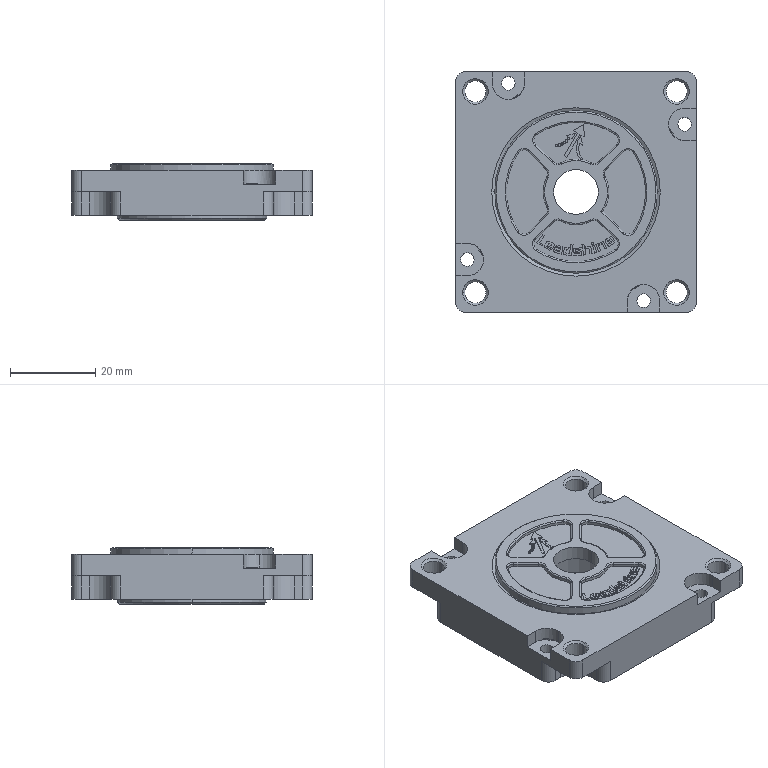Part | SolidWorks | features BaseBody 1 | 1 solid | 382 faces | box 56.4 x 56.4 x 13.3 mm | volume 19484 mm3 | plane 165 | cylinder 101 | spline 100 | cone 16 | commonest cylinder face diameters 0.6 x20 3 x18 4.6 x12 3.2 x8 5 x8 7.6 x5